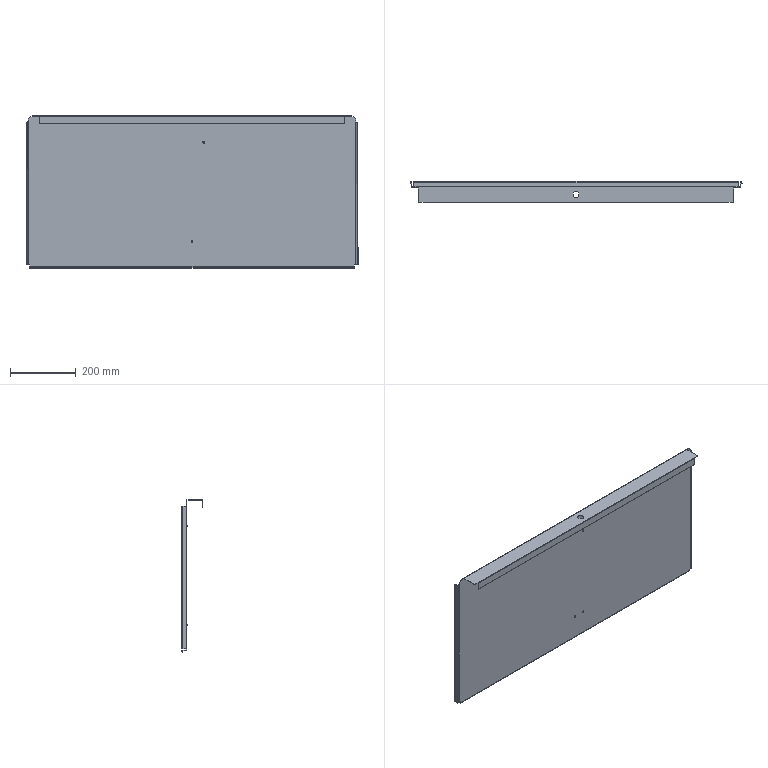Part | SolidWorks | features EdgeFlange 7, ICE 5, RevCut 2, Revolution 2, FlatPattern 1, SM3dBend 1, SMBaseFlange 1, SheetMetal 1 | 1 solid | 96 faces | box 1007 x 66.2 x 462.807 mm | volume 677341 mm3 | plane 63 | cylinder 21 | torus 8 | spline 4 | commonest cylinder face diameters 1 x5 3.4 x5 2 x3 4.4 x3 19.2 x3 40 x2